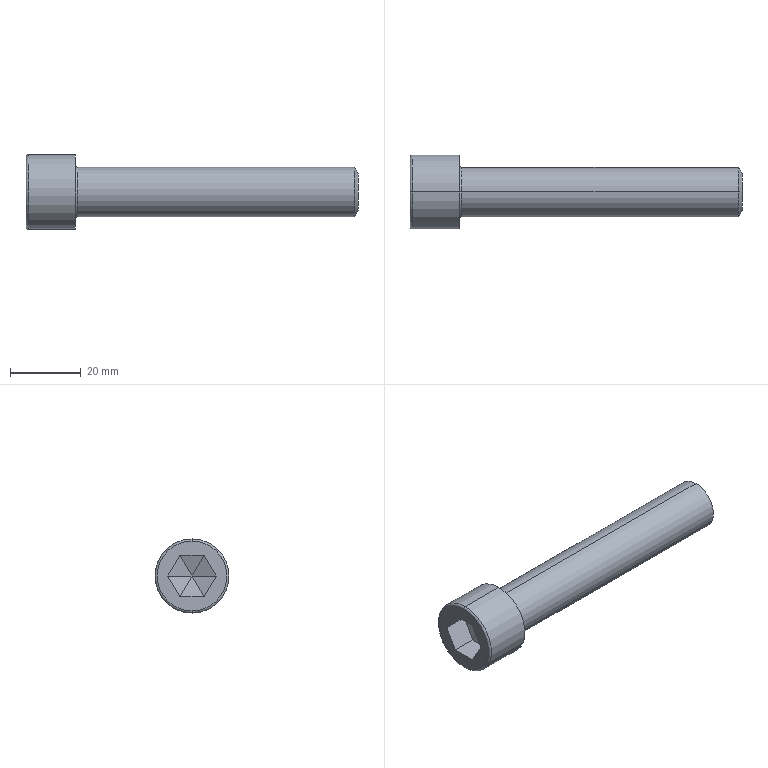Part | SolidWorks | features BlendCut 1, Cut 1, Fillet 1, LPattern 1, RevCut 1, Revolution 1 | 1 solid | 25 faces | box 94 x 21 x 21 mm | volume 16190 mm3 | plane 15 | torus 4 | cylinder 4 | cone 2 | commonest cylinder face diameters 14 x2 21 x2
STEP:
#1=CARTESIAN_POINT('',(94.,0.,5.268));
#2=VERTEX_POINT('',#1);
#3=CARTESIAN_POINT('',(94.,0.,-5.268));
#4=VERTEX_POINT('',#3);
#5=CARTESIAN_POINT('',(94.,0.,0.));
#6=DIRECTION('',(-1.,0.,0.));
#7=DIRECTION('',(0.,0.,1.));
#8=AXIS2_PLACEMENT_3D('',#5,#6,#7);
#9=CIRCLE('',#8,5.268);
#10=EDGE_CURVE('',#2,#4,#9,.T.);
#11=ORIENTED_EDGE('',*,*,#10,.T.);
#12=CARTESIAN_POINT('',(93.,0.,-7.));
#13=VERTEX_POINT('',#12);
#14=CARTESIAN_POINT('',(93.,0.,-7.));
#15=DIRECTION('',(-0.5,0.,-0.866));
#16=VECTOR('',#15,1000.);
#17=LINE('',#14,#16);
#18=EDGE_CURVE('',#4,#13,#17,.T.);
#19=ORIENTED_EDGE('',*,*,#18,.T.);
#20=CARTESIAN_POINT('',(93.,0.,7.));
#21=VERTEX_POINT('',#20);
#22=CARTESIAN_POINT('',(93.,0.,0.));
#23=DIRECTION('',(-1.,0.,0.));
#24=DIRECTION('',(0.,0.,1.));
#25=AXIS2_PLACEMENT_3D('',#22,#23,#24);
#26=CIRCLE('',#25,7.);
#27=EDGE_CURVE('',#21,#13,#26,.T.);
#28=ORIENTED_EDGE('',*,*,#27,.F.);
#29=CARTESIAN_POINT('',(93.,0.,7.));
#30=DIRECTION('',(-0.5,0.,0.866));
#31=VECTOR('',#30,1000.);
#32=LINE('',#29,#31);
#33=EDGE_CURVE('',#2,#21,#32,.T.);
#34=ORIENTED_EDGE('',*,*,#33,.F.);
#35=EDGE_LOOP('',(#11,#19,#28,#34));
#36=FACE_OUTER_BOUND('',#35,.T.);
#37=CARTESIAN_POINT('',(93.,0.,0.));
#38=DIRECTION('',(-1.,0.,0.));
#39=DIRECTION('',(0.,0.,1.));
#40=AXIS2_PLACEMENT_3D('',#37,#38,#39);
#41=CONICAL_SURFACE('',#40,7.,1.047);
#42=ADVANCED_FACE('',(#36),#41,.T.);
#43=CARTESIAN_POINT('',(0.6,0.,-10.5));
#44=VERTEX_POINT('',#43);
#45=CARTESIAN_POINT('',(0.6,0.,10.5));
#46=VERTEX_POINT('',#45);
#47=CARTESIAN_POINT('',(0.6,0.,0.));
#48=DIRECTION('',(1.,0.,0.));
#49=DIRECTION('',(0.,0.,1.));
#50=AXIS2_PLACEMENT_3D('',#47,#48,#49);
#51=CIRCLE('',#50,10.5);
#52=EDGE_CURVE('',#44,#46,#51,.T.);
#53=ORIENTED_EDGE('',*,*,#52,.F.);
#54=CARTESIAN_POINT('',(0.,0.,-9.9));
#55=VERTEX_POINT('',#54);
#56=CARTESIAN_POINT('',(0.6,0.,-9.9));
#57=DIRECTION('',(0.,1.,0.));
#58=DIRECTION('',(0.,0.,1.));
#59=AXIS2_PLACEMENT_3D('',#56,#57,#58);
#60=CIRCLE('',#59,0.6);
#61=EDGE_CURVE('',#44,#55,#60,.T.);
#62=ORIENTED_EDGE('',*,*,#61,.T.);
#63=CARTESIAN_POINT('',(0.,0.,9.9));
#64=VERTEX_POINT('',#63);
#65=CARTESIAN_POINT('',(0.,0.,0.));
#66=DIRECTION('',(-1.,0.,0.));
#67=DIRECTION('',(0.,0.,1.));
#68=AXIS2_PLACEMENT_3D('',#65,#66,#67);
#69=CIRCLE('',#68,9.9);
#70=EDGE_CURVE('',#64,#55,#69,.T.);
#71=ORIENTED_EDGE('',*,*,#70,.F.);
#72=CARTESIAN_POINT('',(0.6,0.,9.9));
#73=DIRECTION('',(0.,-1.,0.));
#74=DIRECTION('',(0.,0.,-1.));
#75=AXIS2_PLACEMENT_3D('',#72,#73,#74);
#76=CIRCLE('',#75,0.6);
#77=EDGE_CURVE('',#46,#64,#76,.T.);
#78=ORIENTED_EDGE('',*,*,#77,.F.);
#79=EDGE_LOOP('',(#53,#62,#71,#78));
#80=FACE_OUTER_BOUND('',#79,.T.);
#81=CARTESIAN_POINT('',(0.6,0.,0.));
#82=DIRECTION('',(-1.,0.,0.));
#83=DIRECTION('',(0.,0.,1.));
#84=AXIS2_PLACEMENT_3D('',#81,#82,#83);
#85=TOROIDAL_SURFACE('',#84,9.9,0.6);
#86=ADVANCED_FACE('',(#80),#85,.T.);
#87=CARTESIAN_POINT('',(14.6,0.,7.));
#88=VERTEX_POINT('',#87);
#89=CARTESIAN_POINT('',(14.6,0.,-7.));
#90=VERTEX_POINT('',#89);
#91=CARTESIAN_POINT('',(14.6,0.,0.));
#92=DIRECTION('',(1.,0.,0.));
#93=DIRECTION('',(0.,0.,-1.));
#94=AXIS2_PLACEMENT_3D('',#91,#92,#93);
#95=CIRCLE('',#94,7.);
#96=EDGE_CURVE('',#88,#90,#95,.T.);
#97=ORIENTED_EDGE('',*,*,#96,.F.);
#98=CARTESIAN_POINT('',(14.,0.,7.6));
#99=VERTEX_POINT('',#98);
#100=CARTESIAN_POINT('',(14.6,0.,7.6));
#101=DIRECTION('',(0.,1.,0.));
#102=DIRECTION('',(0.,0.,1.));
#103=AXIS2_PLACEMENT_3D('',#100,#101,#102);
#104=CIRCLE('',#103,0.6);
#105=EDGE_CURVE('',#88,#99,#104,.T.);
#106=ORIENTED_EDGE('',*,*,#105,.T.);
#107=CARTESIAN_POINT('',(14.,0.,-7.6));
#108=VERTEX_POINT('',#107);
#109=CARTESIAN_POINT('',(14.,0.,0.));
#110=DIRECTION('',(1.,0.,0.));
#111=DIRECTION('',(0.,0.,-1.));
#112=AXIS2_PLACEMENT_3D('',#109,#110,#111);
#113=CIRCLE('',#112,7.6);
#114=EDGE_CURVE('',#99,#108,#113,.T.);
#115=ORIENTED_EDGE('',*,*,#114,.T.);
#116=CARTESIAN_POINT('',(14.6,0.,-7.6));
#117=DIRECTION('',(0.,-1.,0.));
#118=DIRECTION('',(0.,0.,-1.));
#119=AXIS2_PLACEMENT_3D('',#116,#117,#118);
#120=CIRCLE('',#119,0.6);
#121=EDGE_CURVE('',#90,#108,#120,.T.);
#122=ORIENTED_EDGE('',*,*,#121,.F.);
#123=EDGE_LOOP('',(#97,#106,#115,#122));
#124=FACE_OUTER_BOUND('',#123,.T.);
#125=CARTESIAN_POINT('',(14.6,0.,0.));
#126=DIRECTION('',(1.,0.,0.));
#127=DIRECTION('',(0.,0.,-1.));
#128=AXIS2_PLACEMENT_3D('',#125,#126,#127);
#129=TOROIDAL_SURFACE('',#128,7.6,0.6);
#130=ADVANCED_FACE('',(#124),#129,.F.);
#131=ORIENTED_EDGE('',*,*,#52,.T.);
#132=CARTESIAN_POINT('',(14.,0.,10.5));
#133=VERTEX_POINT('',#132);
#134=CARTESIAN_POINT('',(0.,0.,10.5));
#135=DIRECTION('',(1.,0.,0.));
#136=VECTOR('',#135,1000.);
#137=LINE('',#134,#136);
#138=EDGE_CURVE('',#46,#133,#137,.T.);
#139=ORIENTED_EDGE('',*,*,#138,.T.);
#140=CARTESIAN_POINT('',(14.,0.,-10.5));
#141=VERTEX_POINT('',#140);
#142=CARTESIAN_POINT('',(14.,0.,0.));
#143=DIRECTION('',(1.,0.,0.));
#144=DIRECTION('',(0.,0.,-1.));
#145=AXIS2_PLACEMENT_3D('',#142,#143,#144);
#146=CIRCLE('',#145,10.5);
#147=EDGE_CURVE('',#141,#133,#146,.T.);
#148=ORIENTED_EDGE('',*,*,#147,.F.);
#149=CARTESIAN_POINT('',(0.,0.,-10.5));
#150=DIRECTION('',(1.,0.,0.));
#151=VECTOR('',#150,1000.);
#152=LINE('',#149,#151);
#153=EDGE_CURVE('',#44,#141,#152,.T.);
#154=ORIENTED_EDGE('',*,*,#153,.F.);
#155=EDGE_LOOP('',(#131,#139,#148,#154));
#156=FACE_OUTER_BOUND('',#155,.T.);
#157=CARTESIAN_POINT('',(0.,0.,0.));
#158=DIRECTION('',(1.,0.,0.));
#159=DIRECTION('',(0.,0.,-1.));
#160=AXIS2_PLACEMENT_3D('',#157,#158,#159);
#161=CYLINDRICAL_SURFACE('',#160,10.5);
#162=ADVANCED_FACE('',(#156),#161,.T.);
#163=CARTESIAN_POINT('',(14.6,0.,0.));
#164=DIRECTION('',(1.,0.,0.));
#165=DIRECTION('',(0.,0.,-1.));
#166=AXIS2_PLACEMENT_3D('',#163,#164,#165);
#167=CIRCLE('',#166,7.);
#168=EDGE_CURVE('',#90,#88,#167,.T.);
#169=ORIENTED_EDGE('',*,*,#168,.T.);
#170=CARTESIAN_POINT('',(0.,0.,7.));
#171=DIRECTION('',(1.,0.,0.));
#172=VECTOR('',#171,1000.);
#173=LINE('',#170,#172);
#174=EDGE_CURVE('',#88,#21,#173,.T.);
#175=ORIENTED_EDGE('',*,*,#174,.T.);
#176=ORIENTED_EDGE('',*,*,#27,.T.);
#177=CARTESIAN_POINT('',(0.,0.,-7.));
#178=DIRECTION('',(1.,0.,0.));
#179=VECTOR('',#178,1000.);
#180=LINE('',#177,#179);
#181=EDGE_CURVE('',#90,#13,#180,.T.);
#182=ORIENTED_EDGE('',*,*,#181,.F.);
#183=EDGE_LOOP('',(#169,#175,#176,#182));
#184=FACE_OUTER_BOUND('',#183,.T.);
#185=CARTESIAN_POINT('',(0.,0.,0.));
#186=DIRECTION('',(1.,0.,0.));
#187=DIRECTION('',(0.,0.,-1.));
#188=AXIS2_PLACEMENT_3D('',#185,#186,#187);
#189=CYLINDRICAL_SURFACE('',#188,7.);
#190=ADVANCED_FACE('',(#184),#189,.T.);
#191=ORIENTED_EDGE('',*,*,#174,.F.);
#192=ORIENTED_EDGE('',*,*,#96,.T.);
#193=ORIENTED_EDGE('',*,*,#181,.T.);
#194=CARTESIAN_POINT('',(93.,0.,0.));
#195=DIRECTION('',(-1.,0.,0.));
#196=DIRECTION('',(0.,0.,1.));
#197=AXIS2_PLACEMENT_3D('',#194,#195,#196);
#198=CIRCLE('',#197,7.);
#199=EDGE_CURVE('',#13,#21,#198,.T.);
#200=ORIENTED_EDGE('',*,*,#199,.T.);
#201=EDGE_LOOP('',(#191,#192,#193,#200));
#202=FACE_OUTER_BOUND('',#201,.T.);
#203=CARTESIAN_POINT('',(0.,0.,0.));
#204=DIRECTION('',(1.,0.,0.));
#205=DIRECTION('',(0.,0.,-1.));
#206=AXIS2_PLACEMENT_3D('',#203,#204,#205);
#207=CYLINDRICAL_SURFACE('',#206,7.);
#208=ADVANCED_FACE('',(#202),#207,.T.);
#209=ORIENTED_EDGE('',*,*,#70,.T.);
#210=CARTESIAN_POINT('',(0.,0.,0.));
#211=DIRECTION('',(-1.,0.,0.));
#212=DIRECTION('',(0.,0.,1.));
#213=AXIS2_PLACEMENT_3D('',#210,#211,#212);
#214=CIRCLE('',#213,9.9);
#215=EDGE_CURVE('',#55,#64,#214,.T.);
#216=ORIENTED_EDGE('',*,*,#215,.T.);
#217=EDGE_LOOP('',(#209,#216));
#218=FACE_OUTER_BOUND('',#217,.T.);
#219=CARTESIAN_POINT('',(0.,-6.86,0.));
#220=VERTEX_POINT('',#219);
#221=CARTESIAN_POINT('',(0.,-3.43,5.941));
#222=VERTEX_POINT('',#221);
#223=CARTESIAN_POINT('',(0.,-6.86,0.));
#224=DIRECTION('',(0.,0.5,0.866));
#225=VECTOR('',#224,1000.);
#226=LINE('',#223,#225);
#227=EDGE_CURVE('',#220,#222,#226,.T.);
#228=ORIENTED_EDGE('',*,*,#227,.F.);
#229=CARTESIAN_POINT('',(0.,-3.43,-5.941));
#230=VERTEX_POINT('',#229);
#231=CARTESIAN_POINT('',(0.,-3.43,-5.941));
#232=DIRECTION('',(0.,-0.5,0.866));
#233=VECTOR('',#232,1000.);
#234=LINE('',#231,#233);
#235=EDGE_CURVE('',#230,#220,#234,.T.);
#236=ORIENTED_EDGE('',*,*,#235,.F.);
#237=CARTESIAN_POINT('',(0.,3.43,-5.941));
#238=VERTEX_POINT('',#237);
#239=CARTESIAN_POINT('',(0.,3.43,-5.941));
#240=DIRECTION('',(0.,-1.,0.));
#241=VECTOR('',#240,1000.);
#242=LINE('',#239,#241);
#243=EDGE_CURVE('',#238,#230,#242,.T.);
#244=ORIENTED_EDGE('',*,*,#243,.F.);
#245=CARTESIAN_POINT('',(0.,6.86,0.));
#246=VERTEX_POINT('',#245);
#247=CARTESIAN_POINT('',(0.,6.86,0.));
#248=DIRECTION('',(0.,-0.5,-0.866));
#249=VECTOR('',#248,1000.);
#250=LINE('',#247,#249);
#251=EDGE_CURVE('',#246,#238,#250,.T.);
#252=ORIENTED_EDGE('',*,*,#251,.F.);
#253=CARTESIAN_POINT('',(0.,3.43,5.941));
#254=VERTEX_POINT('',#253);
#255=CARTESIAN_POINT('',(0.,3.43,5.941));
#256=DIRECTION('',(0.,0.5,-0.866));
#257=VECTOR('',#256,1000.);
#258=LINE('',#255,#257);
#259=EDGE_CURVE('',#254,#246,#258,.T.);
#260=ORIENTED_EDGE('',*,*,#259,.F.);
#261=CARTESIAN_POINT('',(0.,-3.43,5.941));
#262=DIRECTION('',(0.,1.,0.));
#263=VECTOR('',#262,1000.);
#264=LINE('',#261,#263);
#265=EDGE_CURVE('',#222,#254,#264,.T.);
#266=ORIENTED_EDGE('',*,*,#265,.F.);
#267=EDGE_LOOP('',(#228,#236,#244,#252,#260,#266));
#268=FACE_BOUND('',#267,.T.);
#269=CARTESIAN_POINT('',(0.,0.,0.));
#270=DIRECTION('',(-1.,0.,0.));
#271=DIRECTION('',(0.,0.,1.));
#272=AXIS2_PLACEMENT_3D('',#269,#270,#271);
#273=PLANE('',#272);
#274=ADVANCED_FACE('',(#218,#268),#273,.T.);
#275=ORIENTED_EDGE('',*,*,#138,.F.);
#276=CARTESIAN_POINT('',(0.6,0.,0.));
#277=DIRECTION('',(1.,0.,0.));
#278=DIRECTION('',(0.,0.,1.));
#279=AXIS2_PLACEMENT_3D('',#276,#277,#278);
#280=CIRCLE('',#279,10.5);
#281=EDGE_CURVE('',#46,#44,#280,.T.);
#282=ORIENTED_EDGE('',*,*,#281,.T.);
#283=ORIENTED_EDGE('',*,*,#153,.T.);
#284=CARTESIAN_POINT('',(14.,0.,0.));
#285=DIRECTION('',(1.,0.,0.));
#286=DIRECTION('',(0.,0.,-1.));
#287=AXIS2_PLACEMENT_3D('',#284,#285,#286);
#288=CIRCLE('',#287,10.5);
#289=EDGE_CURVE('',#133,#141,#288,.T.);
#290=ORIENTED_EDGE('',*,*,#289,.F.);
#291=EDGE_LOOP('',(#275,#282,#283,#290));
#292=FACE_OUTER_BOUND('',#291,.T.);
#293=CARTESIAN_POINT('',(0.,0.,0.));
#294=DIRECTION('',(1.,0.,0.));
#295=DIRECTION('',(0.,0.,-1.));
#296=AXIS2_PLACEMENT_3D('',#293,#294,#295);
#297=CYLINDRICAL_SURFACE('',#296,10.5);
#298=ADVANCED_FACE('',(#292),#297,.T.);
#299=ORIENTED_EDGE('',*,*,#147,.T.);
#300=ORIENTED_EDGE('',*,*,#289,.T.);
#301=EDGE_LOOP('',(#299,#300));
#302=FACE_OUTER_BOUND('',#301,.T.);
#303=CARTESIAN_POINT('',(14.,0.,0.));
#304=DIRECTION('',(1.,0.,0.));
#305=DIRECTION('',(0.,0.,-1.));
#306=AXIS2_PLACEMENT_3D('',#303,#304,#305);
#307=CIRCLE('',#306,7.6);
#308=EDGE_CURVE('',#108,#99,#307,.T.);
#309=ORIENTED_EDGE('',*,*,#308,.F.);
#310=ORIENTED_EDGE('',*,*,#114,.F.);
#311=EDGE_LOOP('',(#309,#310));
#312=FACE_BOUND('',#311,.T.);
#313=CARTESIAN_POINT('',(14.,10.5,0.));
#314=DIRECTION('',(1.,0.,0.));
#315=DIRECTION('',(0.,0.,-1.));
#316=AXIS2_PLACEMENT_3D('',#313,#314,#315);
#317=PLANE('',#316);
#318=ADVANCED_FACE('',(#302,#312),#317,.T.);
#319=ORIENTED_EDGE('',*,*,#105,.F.);
#320=ORIENTED_EDGE('',*,*,#168,.F.);
#321=ORIENTED_EDGE('',*,*,#121,.T.);
#322=ORIENTED_EDGE('',*,*,#308,.T.);
#323=EDGE_LOOP('',(#319,#320,#321,#322));
#324=FACE_OUTER_BOUND('',#323,.T.);
#325=CARTESIAN_POINT('',(14.6,0.,0.));
#326=DIRECTION('',(1.,0.,0.));
#327=DIRECTION('',(0.,0.,-1.));
#328=AXIS2_PLACEMENT_3D('',#325,#326,#327);
#329=TOROIDAL_SURFACE('',#328,7.6,0.6);
#330=ADVANCED_FACE('',(#324),#329,.F.);
#331=ORIENTED_EDGE('',*,*,#227,.T.);
#332=CARTESIAN_POINT('',(7.,-3.43,5.941));
#333=VERTEX_POINT('',#332);
#334=CARTESIAN_POINT('',(7.,-3.43,5.941));
#335=DIRECTION('',(-1.,0.,0.));
#336=VECTOR('',#335,1000.);
#337=LINE('',#334,#336);
#338=EDGE_CURVE('',#333,#222,#337,.T.);
#339=ORIENTED_EDGE('',*,*,#338,.F.);
#340=CARTESIAN_POINT('',(7.,-6.86,0.));
#341=VERTEX_POINT('',#340);
#342=CARTESIAN_POINT('',(7.,-6.86,0.));
#343=DIRECTION('',(0.,0.5,0.866));
#344=VECTOR('',#343,1000.);
#345=LINE('',#342,#344);
#346=EDGE_CURVE('',#341,#333,#345,.T.);
#347=ORIENTED_EDGE('',*,*,#346,.F.);
#348=CARTESIAN_POINT('',(7.,-6.86,0.));
#349=DIRECTION('',(-1.,0.,0.));
#350=VECTOR('',#349,1000.);
#351=LINE('',#348,#350);
#352=EDGE_CURVE('',#341,#220,#351,.T.);
#353=ORIENTED_EDGE('',*,*,#352,.T.);
#354=EDGE_LOOP('',(#331,#339,#347,#353));
#355=FACE_OUTER_BOUND('',#354,.T.);
#356=CARTESIAN_POINT('',(7.,-6.86,0.));
#357=DIRECTION('',(0.,-0.866,0.5));
#358=DIRECTION('',(0.,-0.5,-0.866));
#359=AXIS2_PLACEMENT_3D('',#356,#357,#358);
#360=PLANE('',#359);
#361=ADVANCED_FACE('',(#355),#360,.F.);
#362=ORIENTED_EDGE('',*,*,#235,.T.);
#363=ORIENTED_EDGE('',*,*,#352,.F.);
#364=CARTESIAN_POINT('',(7.,-3.43,-5.941));
#365=VERTEX_POINT('',#364);
#366=CARTESIAN_POINT('',(7.,-3.43,-5.941));
#367=DIRECTION('',(0.,-0.5,0.866));
#368=VECTOR('',#367,1000.);
#369=LINE('',#366,#368);
#370=EDGE_CURVE('',#365,#341,#369,.T.);
#371=ORIENTED_EDGE('',*,*,#370,.F.);
#372=CARTESIAN_POINT('',(7.,-3.43,-5.941));
#373=DIRECTION('',(-1.,0.,0.));
#374=VECTOR('',#373,1000.);
#375=LINE('',#372,#374);
#376=EDGE_CURVE('',#365,#230,#375,.T.);
#377=ORIENTED_EDGE('',*,*,#376,.T.);
#378=EDGE_LOOP('',(#362,#363,#371,#377));
#379=FACE_OUTER_BOUND('',#378,.T.);
#380=CARTESIAN_POINT('',(7.,-3.43,-5.941));
#381=DIRECTION('',(0.,-0.866,-0.5));
#382=DIRECTION('',(0.,0.5,-0.866));
#383=AXIS2_PLACEMENT_3D('',#380,#381,#382);
#384=PLANE('',#383);
#385=ADVANCED_FACE('',(#379),#384,.F.);
#386=ORIENTED_EDGE('',*,*,#243,.T.);
#387=ORIENTED_EDGE('',*,*,#376,.F.);
#388=CARTESIAN_POINT('',(7.,3.43,-5.941));
#389=VERTEX_POINT('',#388);
#390=CARTESIAN_POINT('',(7.,3.43,-5.941));
#391=DIRECTION('',(0.,-1.,0.));
#392=VECTOR('',#391,1000.);
#393=LINE('',#390,#392);
#394=EDGE_CURVE('',#389,#365,#393,.T.);
#395=ORIENTED_EDGE('',*,*,#394,.F.);
#396=CARTESIAN_POINT('',(7.,3.43,-5.941));
#397=DIRECTION('',(-1.,0.,0.));
#398=VECTOR('',#397,1000.);
#399=LINE('',#396,#398);
#400=EDGE_CURVE('',#389,#238,#399,.T.);
#401=ORIENTED_EDGE('',*,*,#400,.T.);
#402=EDGE_LOOP('',(#386,#387,#395,#401));
#403=FACE_OUTER_BOUND('',#402,.T.);
#404=CARTESIAN_POINT('',(7.,3.43,-5.941));
#405=DIRECTION('',(0.,0.,-1.));
#406=DIRECTION('',(0.,1.,0.));
#407=AXIS2_PLACEMENT_3D('',#404,#405,#406);
#408=PLANE('',#407);
#409=ADVANCED_FACE('',(#403),#408,.F.);
#410=ORIENTED_EDGE('',*,*,#251,.T.);
#411=ORIENTED_EDGE('',*,*,#400,.F.);
#412=CARTESIAN_POINT('',(7.,6.86,0.));
#413=VERTEX_POINT('',#412);
#414=CARTESIAN_POINT('',(7.,6.86,0.));
#415=DIRECTION('',(0.,-0.5,-0.866));
#416=VECTOR('',#415,1000.);
#417=LINE('',#414,#416);
#418=EDGE_CURVE('',#413,#389,#417,.T.);
#419=ORIENTED_EDGE('',*,*,#418,.F.);
#420=CARTESIAN_POINT('',(7.,6.86,0.));
#421=DIRECTION('',(-1.,0.,0.));
#422=VECTOR('',#421,1000.);
#423=LINE('',#420,#422);
#424=EDGE_CURVE('',#413,#246,#423,.T.);
#425=ORIENTED_EDGE('',*,*,#424,.T.);
#426=EDGE_LOOP('',(#410,#411,#419,#425));
#427=FACE_OUTER_BOUND('',#426,.T.);
#428=CARTESIAN_POINT('',(7.,6.86,0.));
#429=DIRECTION('',(0.,0.866,-0.5));
#430=DIRECTION('',(0.,0.5,0.866));
#431=AXIS2_PLACEMENT_3D('',#428,#429,#430);
#432=PLANE('',#431);
#433=ADVANCED_FACE('',(#427),#432,.F.);
#434=ORIENTED_EDGE('',*,*,#259,.T.);
#435=ORIENTED_EDGE('',*,*,#424,.F.);
#436=CARTESIAN_POINT('',(7.,3.43,5.941));
#437=VERTEX_POINT('',#436);
#438=CARTESIAN_POINT('',(7.,3.43,5.941));
#439=DIRECTION('',(0.,0.5,-0.866));
#440=VECTOR('',#439,1000.);
#441=LINE('',#438,#440);
#442=EDGE_CURVE('',#437,#413,#441,.T.);
#443=ORIENTED_EDGE('',*,*,#442,.F.);
#444=CARTESIAN_POINT('',(7.,3.43,5.941));
#445=DIRECTION('',(-1.,0.,0.));
#446=VECTOR('',#445,1000.);
#447=LINE('',#444,#446);
#448=EDGE_CURVE('',#437,#254,#447,.T.);
#449=ORIENTED_EDGE('',*,*,#448,.T.);
#450=EDGE_LOOP('',(#434,#435,#443,#449));
#451=FACE_OUTER_BOUND('',#450,.T.);
#452=CARTESIAN_POINT('',(7.,3.43,5.941));
#453=DIRECTION('',(0.,0.866,0.5));
#454=DIRECTION('',(0.,-0.5,0.866));
#455=AXIS2_PLACEMENT_3D('',#452,#453,#454);
#456=PLANE('',#455);
#457=ADVANCED_FACE('',(#451),#456,.F.);
#458=ORIENTED_EDGE('',*,*,#265,.T.);
#459=ORIENTED_EDGE('',*,*,#448,.F.);
#460=CARTESIAN_POINT('',(7.,-3.43,5.941));
#461=DIRECTION('',(0.,1.,0.));
#462=VECTOR('',#461,1000.);
#463=LINE('',#460,#462);
#464=EDGE_CURVE('',#333,#437,#463,.T.);
#465=ORIENTED_EDGE('',*,*,#464,.F.);
#466=ORIENTED_EDGE('',*,*,#338,.T.);
#467=EDGE_LOOP('',(#458,#459,#465,#466));
#468=FACE_OUTER_BOUND('',#467,.T.);
#469=CARTESIAN_POINT('',(7.,-3.43,5.941));
#470=DIRECTION('',(0.,0.,1.));
#471=DIRECTION('',(0.,-1.,0.));
#472=AXIS2_PLACEMENT_3D('',#469,#470,#471);
#473=PLANE('',#472);
#474=ADVANCED_FACE('',(#468),#473,.F.);
#475=CARTESIAN_POINT('',(9.,0.,0.));
#476=VERTEX_POINT('',#475);
#477=CARTESIAN_POINT('',(9.,0.,0.));
#478=DIRECTION('',(-0.2799,-0.96,0.));
#479=VECTOR('',#478,1000.);
#480=LINE('',#477,#479);
#481=EDGE_CURVE('',#476,#341,#480,.T.);
#482=ORIENTED_EDGE('',*,*,#481,.F.);
#483=CARTESIAN_POINT('',(9.,0.,0.));
#484=DIRECTION('',(-0.2799,-0.48,-0.8314));
#485=VECTOR('',#484,1000.);
#486=LINE('',#483,#485);
#487=EDGE_CURVE('',#476,#365,#486,.T.);
#488=ORIENTED_EDGE('',*,*,#487,.T.);
#489=ORIENTED_EDGE('',*,*,#370,.T.);
#490=EDGE_LOOP('',(#482,#488,#489));
#491=FACE_OUTER_BOUND('',#490,.T.);
#492=CARTESIAN_POINT('',(7.,-6.86,0.));
#493=DIRECTION('',(-0.9477,0.2763,0.1595));
#494=DIRECTION('',(-0.2799,-0.96,0.));
#495=AXIS2_PLACEMENT_3D('',#492,#493,#494);
#496=PLANE('',#495);
#497=ADVANCED_FACE('',(#491),#496,.T.);
#498=ORIENTED_EDGE('',*,*,#487,.F.);
#499=CARTESIAN_POINT('',(9.,0.,0.));
#500=DIRECTION('',(-0.2799,0.48,-0.8314));
#501=VECTOR('',#500,1000.);
#502=LINE('',#499,#501);
#503=EDGE_CURVE('',#476,#389,#502,.T.);
#504=ORIENTED_EDGE('',*,*,#503,.T.);
#505=ORIENTED_EDGE('',*,*,#394,.T.);
#506=EDGE_LOOP('',(#498,#504,#505));
#507=FACE_OUTER_BOUND('',#506,.T.);
#508=CARTESIAN_POINT('',(7.,-3.43,-5.941));
#509=DIRECTION('',(-0.9477,0.,0.3191));
#510=DIRECTION('',(0.3191,0.,0.9477));
#511=AXIS2_PLACEMENT_3D('',#508,#509,#510);
#512=PLANE('',#511);
#513=ADVANCED_FACE('',(#507),#512,.T.);
#514=CARTESIAN_POINT('',(9.,0.,0.));
#515=DIRECTION('',(-0.2799,-0.48,0.8314));
#516=VECTOR('',#515,1000.);
#517=LINE('',#514,#516);
#518=EDGE_CURVE('',#476,#333,#517,.T.);
#519=ORIENTED_EDGE('',*,*,#518,.F.);
#520=ORIENTED_EDGE('',*,*,#481,.T.);
#521=ORIENTED_EDGE('',*,*,#346,.T.);
#522=EDGE_LOOP('',(#519,#520,#521));
#523=FACE_OUTER_BOUND('',#522,.T.);
#524=CARTESIAN_POINT('',(7.,-3.43,5.941));
#525=DIRECTION('',(-0.9477,0.2763,-0.1595));
#526=DIRECTION('',(-0.2799,-0.96,0.));
#527=AXIS2_PLACEMENT_3D('',#524,#525,#526);
#528=PLANE('',#527);
#529=ADVANCED_FACE('',(#523),#528,.T.);
#530=ORIENTED_EDGE('',*,*,#503,.F.);
#531=CARTESIAN_POINT('',(9.,0.,0.));
#532=DIRECTION('',(-0.2799,0.96,0.));
#533=VECTOR('',#532,1000.);
#534=LINE('',#531,#533);
#535=EDGE_CURVE('',#476,#413,#534,.T.);
#536=ORIENTED_EDGE('',*,*,#535,.T.);
#537=ORIENTED_EDGE('',*,*,#418,.T.);
#538=EDGE_LOOP('',(#530,#536,#537));
#539=FACE_OUTER_BOUND('',#538,.T.);
#540=CARTESIAN_POINT('',(7.,3.43,-5.941));
#541=DIRECTION('',(-0.9477,-0.2763,0.1595));
#542=DIRECTION('',(0.2799,-0.96,0.));
#543=AXIS2_PLACEMENT_3D('',#540,#541,#542);
#544=PLANE('',#543);
#545=ADVANCED_FACE('',(#539),#544,.T.);
#546=CARTESIAN_POINT('',(9.,0.,0.));
#547=DIRECTION('',(-0.2799,0.48,0.8314));
#548=VECTOR('',#547,1000.);
#549=LINE('',#546,#548);
#550=EDGE_CURVE('',#476,#437,#549,.T.);
#551=ORIENTED_EDGE('',*,*,#550,.F.);
#552=ORIENTED_EDGE('',*,*,#518,.T.);
#553=ORIENTED_EDGE('',*,*,#464,.T.);
#554=EDGE_LOOP('',(#551,#552,#553));
#555=FACE_OUTER_BOUND('',#554,.T.);
#556=CARTESIAN_POINT('',(7.,3.43,5.941));
#557=DIRECTION('',(-0.9477,0.,-0.3191));
#558=DIRECTION('',(-0.3191,0.,0.9477));
#559=AXIS2_PLACEMENT_3D('',#556,#557,#558);
#560=PLANE('',#559);
#561=ADVANCED_FACE('',(#555),#560,.T.);
#562=ORIENTED_EDGE('',*,*,#535,.F.);
#563=ORIENTED_EDGE('',*,*,#550,.T.);
#564=ORIENTED_EDGE('',*,*,#442,.T.);
#565=EDGE_LOOP('',(#562,#563,#564));
#566=FACE_OUTER_BOUND('',#565,.T.);
#567=CARTESIAN_POINT('',(7.,6.86,0.));
#568=DIRECTION('',(-0.9477,-0.2763,-0.1595));
#569=DIRECTION('',(0.2799,-0.96,0.));
#570=AXIS2_PLACEMENT_3D('',#567,#568,#569);
#571=PLANE('',#570);
#572=ADVANCED_FACE('',(#566),#571,.T.);
#573=ORIENTED_EDGE('',*,*,#61,.F.);
#574=ORIENTED_EDGE('',*,*,#281,.F.);
#575=ORIENTED_EDGE('',*,*,#77,.T.);
#576=ORIENTED_EDGE('',*,*,#215,.F.);
#577=EDGE_LOOP('',(#573,#574,#575,#576));
#578=FACE_OUTER_BOUND('',#577,.T.);
#579=CARTESIAN_POINT('',(0.6,0.,0.));
#580=DIRECTION('',(-1.,0.,0.));
#581=DIRECTION('',(0.,0.,1.));
#582=AXIS2_PLACEMENT_3D('',#579,#580,#581);
#583=TOROIDAL_SURFACE('',#582,9.9,0.6);
#584=ADVANCED_FACE('',(#578),#583,.T.);
#585=ORIENTED_EDGE('',*,*,#18,.F.);
#586=CARTESIAN_POINT('',(94.,0.,0.));
#587=DIRECTION('',(-1.,0.,0.));
#588=DIRECTION('',(0.,0.,1.));
#589=AXIS2_PLACEMENT_3D('',#586,#587,#588);
#590=CIRCLE('',#589,5.268);
#591=EDGE_CURVE('',#4,#2,#590,.T.);
#592=ORIENTED_EDGE('',*,*,#591,.T.);
#593=ORIENTED_EDGE('',*,*,#33,.T.);
#594=ORIENTED_EDGE('',*,*,#199,.F.);
#595=EDGE_LOOP('',(#585,#592,#593,#594));
#596=FACE_OUTER_BOUND('',#595,.T.);
#597=CARTESIAN_POINT('',(93.,0.,0.));
#598=DIRECTION('',(-1.,0.,0.));
#599=DIRECTION('',(0.,0.,1.));
#600=AXIS2_PLACEMENT_3D('',#597,#598,#599);
#601=CONICAL_SURFACE('',#600,7.,1.047);
#602=ADVANCED_FACE('',(#596),#601,.T.);
#603=ORIENTED_EDGE('',*,*,#10,.F.);
#604=ORIENTED_EDGE('',*,*,#591,.F.);
#605=EDGE_LOOP('',(#603,#604));
#606=FACE_OUTER_BOUND('',#605,.T.);
#607=CARTESIAN_POINT('',(94.,7.,0.));
#608=DIRECTION('',(1.,0.,0.));
#609=DIRECTION('',(0.,0.,-1.));
#610=AXIS2_PLACEMENT_3D('',#607,#608,#609);
#611=PLANE('',#610);
#612=ADVANCED_FACE('',(#606),#611,.T.);
#613=CLOSED_SHELL('',(#42,#86,#130,#162,#190,#208,#274,#298,#318,#330,#361,#385,#409,#433,#457,#474,#497,#513,#529,#545,#561,#572,#584,#602,#612));
#614=MANIFOLD_SOLID_BREP('',#613);
#615=CARTESIAN_POINT('',(0.,0.,0.));
#616=DIRECTION('',(0.,0.,1.));
#617=DIRECTION('',(1.,0.,0.));
#618=AXIS2_PLACEMENT_3D('',#615,#616,#617);
#619=(LENGTH_UNIT()NAMED_UNIT(*)SI_UNIT(.MILLI.,.METRE.));
#620=UNCERTAINTY_MEASURE_WITH_UNIT(LENGTH_MEASURE(0.00001),#619,'','');
#621=(NAMED_UNIT(*)PLANE_ANGLE_UNIT()SI_UNIT($,.RADIAN.));
#622=(NAMED_UNIT(*)SI_UNIT($,.STERADIAN.)SOLID_ANGLE_UNIT());
#623=(GEOMETRIC_REPRESENTATION_CONTEXT(3)GLOBAL_UNCERTAINTY_ASSIGNED_CONTEXT((#620))GLOBAL_UNIT_ASSIGNED_CONTEXT((#619,#621,#622))REPRESENTATION_CONTEXT('',''));
#624=ADVANCED_BREP_SHAPE_REPRESENTATION('',(#614,#618),#623);